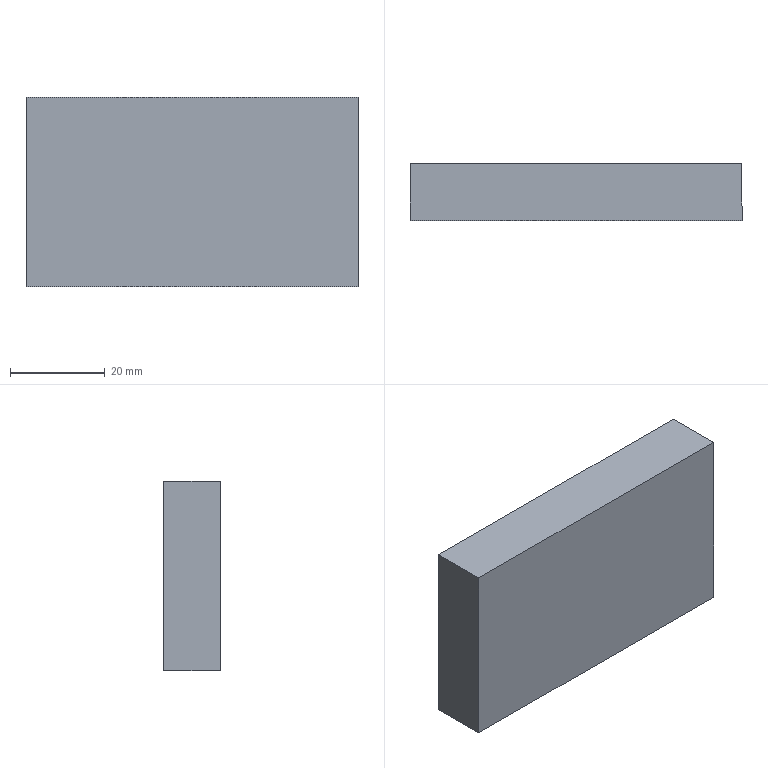Part | STEP file | 手指气缸座-2 | 1 solid | 6 faces | box 70 x 12 x 40 mm | volume 33600 mm3 | plane 6
STEP:
#1=CARTESIAN_POINT('',(-35.,79.,0.));
#2=VERTEX_POINT('',#1);
#3=CARTESIAN_POINT('',(-35.,67.,0.));
#4=VERTEX_POINT('',#3);
#5=CARTESIAN_POINT('',(-35.,79.,0.));
#6=DIRECTION('',(0.,-1.,0.));
#7=VECTOR('',#6,1000.);
#8=LINE('',#5,#7);
#9=EDGE_CURVE('',#2,#4,#8,.T.);
#10=ORIENTED_EDGE('',*,*,#9,.T.);
#11=CARTESIAN_POINT('',(-35.,67.,40.));
#12=VERTEX_POINT('',#11);
#13=CARTESIAN_POINT('',(-35.,67.,40.));
#14=DIRECTION('',(0.,0.,-1.));
#15=VECTOR('',#14,1000.);
#16=LINE('',#13,#15);
#17=EDGE_CURVE('',#12,#4,#16,.T.);
#18=ORIENTED_EDGE('',*,*,#17,.F.);
#19=CARTESIAN_POINT('',(-35.,79.,40.));
#20=VERTEX_POINT('',#19);
#21=CARTESIAN_POINT('',(-35.,79.,40.));
#22=DIRECTION('',(0.,-1.,0.));
#23=VECTOR('',#22,1000.);
#24=LINE('',#21,#23);
#25=EDGE_CURVE('',#20,#12,#24,.T.);
#26=ORIENTED_EDGE('',*,*,#25,.F.);
#27=CARTESIAN_POINT('',(-35.,79.,40.));
#28=DIRECTION('',(0.,0.,-1.));
#29=VECTOR('',#28,1000.);
#30=LINE('',#27,#29);
#31=EDGE_CURVE('',#20,#2,#30,.T.);
#32=ORIENTED_EDGE('',*,*,#31,.T.);
#33=EDGE_LOOP('',(#10,#18,#26,#32));
#34=FACE_OUTER_BOUND('',#33,.T.);
#35=CARTESIAN_POINT('',(-35.,79.,40.));
#36=DIRECTION('',(1.,0.,0.));
#37=DIRECTION('',(0.,0.,-1.));
#38=AXIS2_PLACEMENT_3D('',#35,#36,#37);
#39=PLANE('',#38);
#40=ADVANCED_FACE('',(#34),#39,.F.);
#41=CARTESIAN_POINT('',(35.,67.,0.));
#42=VERTEX_POINT('',#41);
#43=CARTESIAN_POINT('',(-35.,67.,0.));
#44=DIRECTION('',(1.,0.,0.));
#45=VECTOR('',#44,1000.);
#46=LINE('',#43,#45);
#47=EDGE_CURVE('',#4,#42,#46,.T.);
#48=ORIENTED_EDGE('',*,*,#47,.T.);
#49=CARTESIAN_POINT('',(35.,67.,40.));
#50=VERTEX_POINT('',#49);
#51=CARTESIAN_POINT('',(35.,67.,40.));
#52=DIRECTION('',(0.,0.,-1.));
#53=VECTOR('',#52,1000.);
#54=LINE('',#51,#53);
#55=EDGE_CURVE('',#50,#42,#54,.T.);
#56=ORIENTED_EDGE('',*,*,#55,.F.);
#57=CARTESIAN_POINT('',(-35.,67.,40.));
#58=DIRECTION('',(1.,0.,0.));
#59=VECTOR('',#58,1000.);
#60=LINE('',#57,#59);
#61=EDGE_CURVE('',#12,#50,#60,.T.);
#62=ORIENTED_EDGE('',*,*,#61,.F.);
#63=ORIENTED_EDGE('',*,*,#17,.T.);
#64=EDGE_LOOP('',(#48,#56,#62,#63));
#65=FACE_OUTER_BOUND('',#64,.T.);
#66=CARTESIAN_POINT('',(-35.,67.,40.));
#67=DIRECTION('',(0.,1.,0.));
#68=DIRECTION('',(0.,0.,1.));
#69=AXIS2_PLACEMENT_3D('',#66,#67,#68);
#70=PLANE('',#69);
#71=ADVANCED_FACE('',(#65),#70,.F.);
#72=CARTESIAN_POINT('',(35.,79.,0.));
#73=VERTEX_POINT('',#72);
#74=CARTESIAN_POINT('',(35.,79.,0.));
#75=DIRECTION('',(0.,1.,0.));
#76=VECTOR('',#75,1000.);
#77=LINE('',#74,#76);
#78=EDGE_CURVE('',#42,#73,#77,.T.);
#79=ORIENTED_EDGE('',*,*,#78,.T.);
#80=CARTESIAN_POINT('',(35.,79.,40.));
#81=VERTEX_POINT('',#80);
#82=CARTESIAN_POINT('',(35.,79.,40.));
#83=DIRECTION('',(0.,0.,-1.));
#84=VECTOR('',#83,1000.);
#85=LINE('',#82,#84);
#86=EDGE_CURVE('',#81,#73,#85,.T.);
#87=ORIENTED_EDGE('',*,*,#86,.F.);
#88=CARTESIAN_POINT('',(35.,79.,40.));
#89=DIRECTION('',(0.,1.,0.));
#90=VECTOR('',#89,1000.);
#91=LINE('',#88,#90);
#92=EDGE_CURVE('',#50,#81,#91,.T.);
#93=ORIENTED_EDGE('',*,*,#92,.F.);
#94=ORIENTED_EDGE('',*,*,#55,.T.);
#95=EDGE_LOOP('',(#79,#87,#93,#94));
#96=FACE_OUTER_BOUND('',#95,.T.);
#97=CARTESIAN_POINT('',(35.,79.,40.));
#98=DIRECTION('',(-1.,0.,0.));
#99=DIRECTION('',(0.,-1.,0.));
#100=AXIS2_PLACEMENT_3D('',#97,#98,#99);
#101=PLANE('',#100);
#102=ADVANCED_FACE('',(#96),#101,.F.);
#103=CARTESIAN_POINT('',(-35.,79.,0.));
#104=DIRECTION('',(-1.,0.,0.));
#105=VECTOR('',#104,1000.);
#106=LINE('',#103,#105);
#107=EDGE_CURVE('',#73,#2,#106,.T.);
#108=ORIENTED_EDGE('',*,*,#107,.T.);
#109=ORIENTED_EDGE('',*,*,#31,.F.);
#110=CARTESIAN_POINT('',(-35.,79.,40.));
#111=DIRECTION('',(-1.,0.,0.));
#112=VECTOR('',#111,1000.);
#113=LINE('',#110,#112);
#114=EDGE_CURVE('',#81,#20,#113,.T.);
#115=ORIENTED_EDGE('',*,*,#114,.F.);
#116=ORIENTED_EDGE('',*,*,#86,.T.);
#117=EDGE_LOOP('',(#108,#109,#115,#116));
#118=FACE_OUTER_BOUND('',#117,.T.);
#119=CARTESIAN_POINT('',(-35.,79.,40.));
#120=DIRECTION('',(0.,-1.,0.));
#121=DIRECTION('',(0.,0.,-1.));
#122=AXIS2_PLACEMENT_3D('',#119,#120,#121);
#123=PLANE('',#122);
#124=ADVANCED_FACE('',(#118),#123,.F.);
#125=ORIENTED_EDGE('',*,*,#25,.T.);
#126=ORIENTED_EDGE('',*,*,#61,.T.);
#127=ORIENTED_EDGE('',*,*,#92,.T.);
#128=ORIENTED_EDGE('',*,*,#114,.T.);
#129=EDGE_LOOP('',(#125,#126,#127,#128));
#130=FACE_OUTER_BOUND('',#129,.T.);
#131=CARTESIAN_POINT('',(-35.,67.,40.));
#132=DIRECTION('',(0.,0.,1.));
#133=DIRECTION('',(1.,0.,0.));
#134=AXIS2_PLACEMENT_3D('',#131,#132,#133);
#135=PLANE('',#134);
#136=ADVANCED_FACE('',(#130),#135,.T.);
#137=ORIENTED_EDGE('',*,*,#9,.F.);
#138=ORIENTED_EDGE('',*,*,#107,.F.);
#139=ORIENTED_EDGE('',*,*,#78,.F.);
#140=ORIENTED_EDGE('',*,*,#47,.F.);
#141=EDGE_LOOP('',(#137,#138,#139,#140));
#142=FACE_OUTER_BOUND('',#141,.T.);
#143=CARTESIAN_POINT('',(-35.,67.,0.));
#144=DIRECTION('',(0.,0.,1.));
#145=DIRECTION('',(1.,0.,0.));
#146=AXIS2_PLACEMENT_3D('',#143,#144,#145);
#147=PLANE('',#146);
#148=ADVANCED_FACE('',(#142),#147,.F.);
#149=CLOSED_SHELL('',(#40,#71,#102,#124,#136,#148));
#150=MANIFOLD_SOLID_BREP('',#149);
#151=CARTESIAN_POINT('',(0.,0.,0.));
#152=DIRECTION('',(0.,0.,1.));
#153=DIRECTION('',(1.,0.,0.));
#154=AXIS2_PLACEMENT_3D('',#151,#152,#153);
#155=(LENGTH_UNIT()NAMED_UNIT(*)SI_UNIT(.MILLI.,.METRE.));
#156=UNCERTAINTY_MEASURE_WITH_UNIT(LENGTH_MEASURE(0.00001),#155,'','');
#157=(NAMED_UNIT(*)PLANE_ANGLE_UNIT()SI_UNIT($,.RADIAN.));
#158=(NAMED_UNIT(*)SI_UNIT($,.STERADIAN.)SOLID_ANGLE_UNIT());
#159=(GEOMETRIC_REPRESENTATION_CONTEXT(3)GLOBAL_UNCERTAINTY_ASSIGNED_CONTEXT((#156))GLOBAL_UNIT_ASSIGNED_CONTEXT((#155,#157,#158))REPRESENTATION_CONTEXT('',''));
#160=ADVANCED_BREP_SHAPE_REPRESENTATION('',(#150,#154),#159);